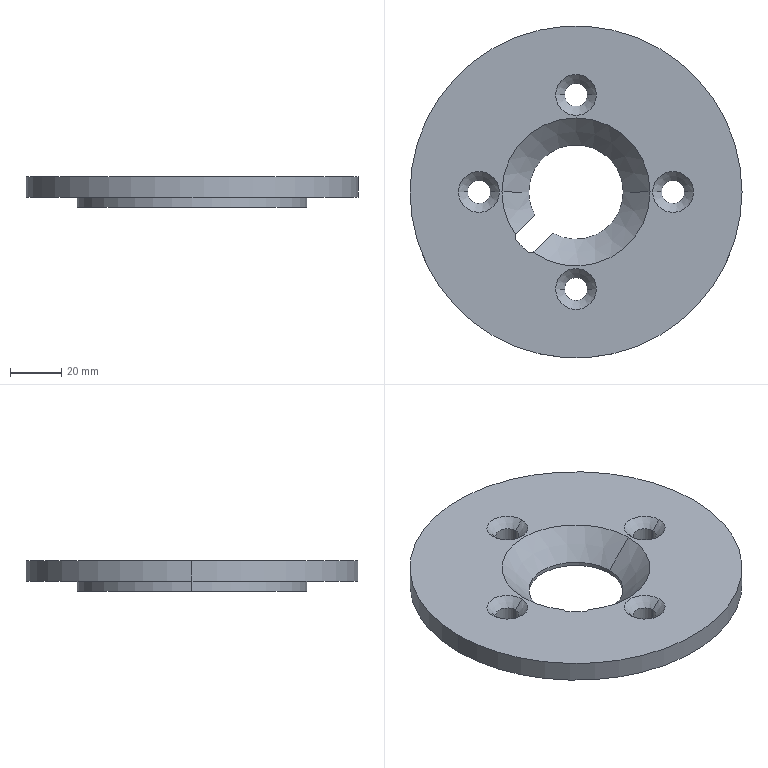Part | STEP file | PCA-130120 | 1 solid | 36 faces | box 130 x 130 x 12 mm | volume 106365 mm3 | cylinder 20 | cone 11 | plane 5 | commonest cylinder face diameters 9 x8 37 x3 2 x2 4 x2 90 x2 130 x2